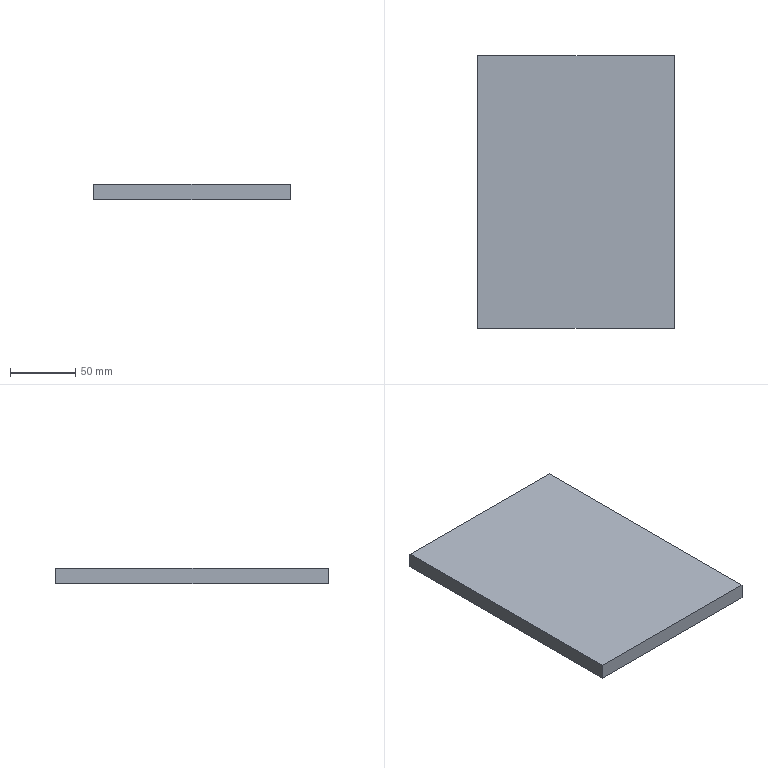Part | SolidWorks | features Extrusion 1 | 1 solid | 6 faces | box 151 x 209 x 12 mm | volume 378708 mm3 | plane 6
STEP:
#1=CARTESIAN_POINT('',(-75.5,104.5,0.));
#2=VERTEX_POINT('',#1);
#3=CARTESIAN_POINT('',(-75.5,-104.5,0.));
#4=VERTEX_POINT('',#3);
#5=CARTESIAN_POINT('',(-75.5,104.5,0.));
#6=DIRECTION('',(0.,-1.,0.));
#7=VECTOR('',#6,1000.);
#8=LINE('',#5,#7);
#9=EDGE_CURVE('',#2,#4,#8,.T.);
#10=ORIENTED_EDGE('',*,*,#9,.T.);
#11=CARTESIAN_POINT('',(-75.5,-104.5,12.));
#12=VERTEX_POINT('',#11);
#13=CARTESIAN_POINT('',(-75.5,-104.5,12.));
#14=DIRECTION('',(0.,0.,-1.));
#15=VECTOR('',#14,1000.);
#16=LINE('',#13,#15);
#17=EDGE_CURVE('',#12,#4,#16,.T.);
#18=ORIENTED_EDGE('',*,*,#17,.F.);
#19=CARTESIAN_POINT('',(-75.5,104.5,12.));
#20=VERTEX_POINT('',#19);
#21=CARTESIAN_POINT('',(-75.5,104.5,12.));
#22=DIRECTION('',(0.,-1.,0.));
#23=VECTOR('',#22,1000.);
#24=LINE('',#21,#23);
#25=EDGE_CURVE('',#20,#12,#24,.T.);
#26=ORIENTED_EDGE('',*,*,#25,.F.);
#27=CARTESIAN_POINT('',(-75.5,104.5,12.));
#28=DIRECTION('',(0.,0.,-1.));
#29=VECTOR('',#28,1000.);
#30=LINE('',#27,#29);
#31=EDGE_CURVE('',#20,#2,#30,.T.);
#32=ORIENTED_EDGE('',*,*,#31,.T.);
#33=EDGE_LOOP('',(#10,#18,#26,#32));
#34=FACE_OUTER_BOUND('',#33,.T.);
#35=CARTESIAN_POINT('',(-75.5,104.5,12.));
#36=DIRECTION('',(1.,0.,0.));
#37=DIRECTION('',(0.,0.,-1.));
#38=AXIS2_PLACEMENT_3D('',#35,#36,#37);
#39=PLANE('',#38);
#40=ADVANCED_FACE('',(#34),#39,.F.);
#41=CARTESIAN_POINT('',(75.5,-104.5,0.));
#42=VERTEX_POINT('',#41);
#43=CARTESIAN_POINT('',(75.5,-104.5,0.));
#44=DIRECTION('',(1.,0.,0.));
#45=VECTOR('',#44,1000.);
#46=LINE('',#43,#45);
#47=EDGE_CURVE('',#4,#42,#46,.T.);
#48=ORIENTED_EDGE('',*,*,#47,.T.);
#49=CARTESIAN_POINT('',(75.5,-104.5,12.));
#50=VERTEX_POINT('',#49);
#51=CARTESIAN_POINT('',(75.5,-104.5,12.));
#52=DIRECTION('',(0.,0.,-1.));
#53=VECTOR('',#52,1000.);
#54=LINE('',#51,#53);
#55=EDGE_CURVE('',#50,#42,#54,.T.);
#56=ORIENTED_EDGE('',*,*,#55,.F.);
#57=CARTESIAN_POINT('',(75.5,-104.5,12.));
#58=DIRECTION('',(1.,0.,0.));
#59=VECTOR('',#58,1000.);
#60=LINE('',#57,#59);
#61=EDGE_CURVE('',#12,#50,#60,.T.);
#62=ORIENTED_EDGE('',*,*,#61,.F.);
#63=ORIENTED_EDGE('',*,*,#17,.T.);
#64=EDGE_LOOP('',(#48,#56,#62,#63));
#65=FACE_OUTER_BOUND('',#64,.T.);
#66=CARTESIAN_POINT('',(75.5,-104.5,12.));
#67=DIRECTION('',(0.,1.,0.));
#68=DIRECTION('',(-1.,0.,0.));
#69=AXIS2_PLACEMENT_3D('',#66,#67,#68);
#70=PLANE('',#69);
#71=ADVANCED_FACE('',(#65),#70,.F.);
#72=CARTESIAN_POINT('',(75.5,104.5,0.));
#73=VERTEX_POINT('',#72);
#74=CARTESIAN_POINT('',(75.5,104.5,0.));
#75=DIRECTION('',(0.,1.,0.));
#76=VECTOR('',#75,1000.);
#77=LINE('',#74,#76);
#78=EDGE_CURVE('',#42,#73,#77,.T.);
#79=ORIENTED_EDGE('',*,*,#78,.T.);
#80=CARTESIAN_POINT('',(75.5,104.5,12.));
#81=VERTEX_POINT('',#80);
#82=CARTESIAN_POINT('',(75.5,104.5,12.));
#83=DIRECTION('',(0.,0.,-1.));
#84=VECTOR('',#83,1000.);
#85=LINE('',#82,#84);
#86=EDGE_CURVE('',#81,#73,#85,.T.);
#87=ORIENTED_EDGE('',*,*,#86,.F.);
#88=CARTESIAN_POINT('',(75.5,104.5,12.));
#89=DIRECTION('',(0.,1.,0.));
#90=VECTOR('',#89,1000.);
#91=LINE('',#88,#90);
#92=EDGE_CURVE('',#50,#81,#91,.T.);
#93=ORIENTED_EDGE('',*,*,#92,.F.);
#94=ORIENTED_EDGE('',*,*,#55,.T.);
#95=EDGE_LOOP('',(#79,#87,#93,#94));
#96=FACE_OUTER_BOUND('',#95,.T.);
#97=CARTESIAN_POINT('',(75.5,104.5,12.));
#98=DIRECTION('',(-1.,0.,0.));
#99=DIRECTION('',(0.,-1.,0.));
#100=AXIS2_PLACEMENT_3D('',#97,#98,#99);
#101=PLANE('',#100);
#102=ADVANCED_FACE('',(#96),#101,.F.);
#103=CARTESIAN_POINT('',(75.5,104.5,0.));
#104=DIRECTION('',(-1.,0.,0.));
#105=VECTOR('',#104,1000.);
#106=LINE('',#103,#105);
#107=EDGE_CURVE('',#73,#2,#106,.T.);
#108=ORIENTED_EDGE('',*,*,#107,.T.);
#109=ORIENTED_EDGE('',*,*,#31,.F.);
#110=CARTESIAN_POINT('',(75.5,104.5,12.));
#111=DIRECTION('',(-1.,0.,0.));
#112=VECTOR('',#111,1000.);
#113=LINE('',#110,#112);
#114=EDGE_CURVE('',#81,#20,#113,.T.);
#115=ORIENTED_EDGE('',*,*,#114,.F.);
#116=ORIENTED_EDGE('',*,*,#86,.T.);
#117=EDGE_LOOP('',(#108,#109,#115,#116));
#118=FACE_OUTER_BOUND('',#117,.T.);
#119=CARTESIAN_POINT('',(75.5,104.5,12.));
#120=DIRECTION('',(0.,-1.,0.));
#121=DIRECTION('',(0.,0.,-1.));
#122=AXIS2_PLACEMENT_3D('',#119,#120,#121);
#123=PLANE('',#122);
#124=ADVANCED_FACE('',(#118),#123,.F.);
#125=ORIENTED_EDGE('',*,*,#25,.T.);
#126=ORIENTED_EDGE('',*,*,#61,.T.);
#127=ORIENTED_EDGE('',*,*,#92,.T.);
#128=ORIENTED_EDGE('',*,*,#114,.T.);
#129=EDGE_LOOP('',(#125,#126,#127,#128));
#130=FACE_OUTER_BOUND('',#129,.T.);
#131=CARTESIAN_POINT('',(0.,0.,12.));
#132=DIRECTION('',(0.,0.,-1.));
#133=DIRECTION('',(-1.,0.,0.));
#134=AXIS2_PLACEMENT_3D('',#131,#132,#133);
#135=PLANE('',#134);
#136=ADVANCED_FACE('',(#130),#135,.F.);
#137=ORIENTED_EDGE('',*,*,#9,.F.);
#138=ORIENTED_EDGE('',*,*,#107,.F.);
#139=ORIENTED_EDGE('',*,*,#78,.F.);
#140=ORIENTED_EDGE('',*,*,#47,.F.);
#141=EDGE_LOOP('',(#137,#138,#139,#140));
#142=FACE_OUTER_BOUND('',#141,.T.);
#143=CARTESIAN_POINT('',(0.,0.,0.));
#144=DIRECTION('',(0.,0.,-1.));
#145=DIRECTION('',(-1.,0.,0.));
#146=AXIS2_PLACEMENT_3D('',#143,#144,#145);
#147=PLANE('',#146);
#148=ADVANCED_FACE('',(#142),#147,.T.);
#149=CLOSED_SHELL('',(#40,#71,#102,#124,#136,#148));
#150=MANIFOLD_SOLID_BREP('',#149);
#151=CARTESIAN_POINT('',(0.,0.,0.));
#152=DIRECTION('',(0.,0.,1.));
#153=DIRECTION('',(1.,0.,0.));
#154=AXIS2_PLACEMENT_3D('',#151,#152,#153);
#155=(LENGTH_UNIT()NAMED_UNIT(*)SI_UNIT(.MILLI.,.METRE.));
#156=UNCERTAINTY_MEASURE_WITH_UNIT(LENGTH_MEASURE(0.00001),#155,'','');
#157=(NAMED_UNIT(*)PLANE_ANGLE_UNIT()SI_UNIT($,.RADIAN.));
#158=(NAMED_UNIT(*)SI_UNIT($,.STERADIAN.)SOLID_ANGLE_UNIT());
#159=(GEOMETRIC_REPRESENTATION_CONTEXT(3)GLOBAL_UNCERTAINTY_ASSIGNED_CONTEXT((#156))GLOBAL_UNIT_ASSIGNED_CONTEXT((#155,#157,#158))REPRESENTATION_CONTEXT('',''));
#160=ADVANCED_BREP_SHAPE_REPRESENTATION('',(#150,#154),#159);